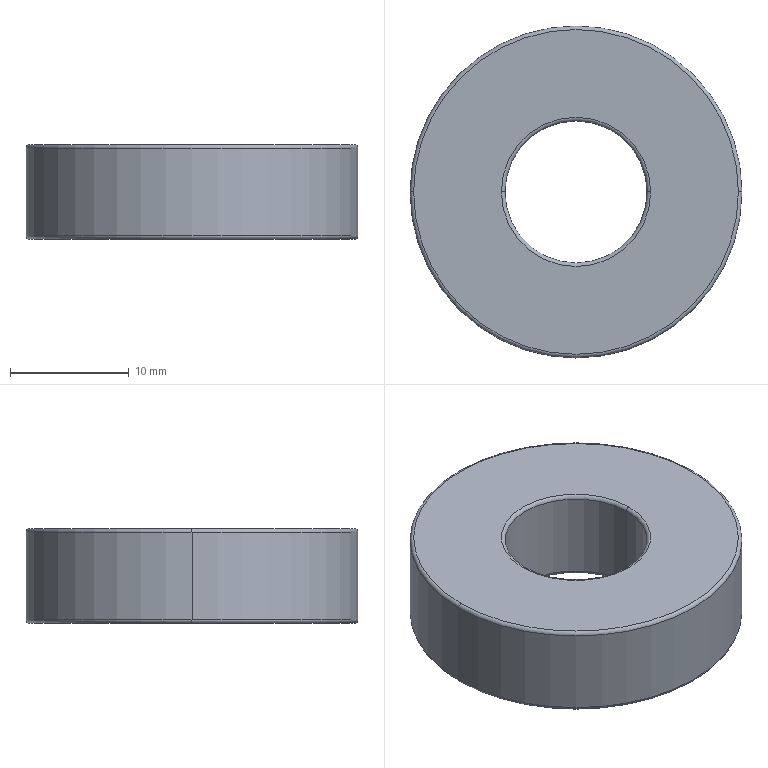Part | SolidWorks | features BaseBody 1 | 1 solid | 14 faces | box 28 x 28 x 8 mm | volume 4016 mm3 | torus 8 | cylinder 4 | plane 2 | commonest cylinder face diameters 12 x2 28 x2
STEP:
#1=CARTESIAN_POINT('',(-14.,0.,3.7));
#2=VERTEX_POINT('',#1);
#3=CARTESIAN_POINT('',(14.,0.,3.7));
#4=VERTEX_POINT('',#3);
#5=CARTESIAN_POINT('',(0.,0.,3.7));
#6=DIRECTION('',(0.,0.,-1.));
#7=DIRECTION('',(1.,0.,0.));
#8=AXIS2_PLACEMENT_3D('',#5,#6,#7);
#9=CIRCLE('',#8,14.);
#10=EDGE_CURVE('',#2,#4,#9,.T.);
#11=ORIENTED_EDGE('',*,*,#10,.F.);
#12=CARTESIAN_POINT('',(-13.7,0.,4.));
#13=VERTEX_POINT('',#12);
#14=CARTESIAN_POINT('',(-13.7,0.,3.7));
#15=DIRECTION('',(0.,1.,0.));
#16=DIRECTION('',(-1.,0.,0.));
#17=AXIS2_PLACEMENT_3D('',#14,#15,#16);
#18=CIRCLE('',#17,0.3);
#19=EDGE_CURVE('',#2,#13,#18,.T.);
#20=ORIENTED_EDGE('',*,*,#19,.T.);
#21=CARTESIAN_POINT('',(13.7,0.,4.));
#22=VERTEX_POINT('',#21);
#23=CARTESIAN_POINT('',(0.,0.,4.));
#24=DIRECTION('',(0.,0.,1.));
#25=DIRECTION('',(1.,0.,0.));
#26=AXIS2_PLACEMENT_3D('',#23,#24,#25);
#27=CIRCLE('',#26,13.7);
#28=EDGE_CURVE('',#22,#13,#27,.T.);
#29=ORIENTED_EDGE('',*,*,#28,.F.);
#30=CARTESIAN_POINT('',(13.7,0.,3.7));
#31=DIRECTION('',(0.,-1.,0.));
#32=DIRECTION('',(0.,0.,-1.));
#33=AXIS2_PLACEMENT_3D('',#30,#31,#32);
#34=CIRCLE('',#33,0.3);
#35=EDGE_CURVE('',#4,#22,#34,.T.);
#36=ORIENTED_EDGE('',*,*,#35,.F.);
#37=EDGE_LOOP('',(#11,#20,#29,#36));
#38=FACE_OUTER_BOUND('',#37,.T.);
#39=CARTESIAN_POINT('',(0.,0.,3.7));
#40=DIRECTION('',(0.,0.,1.));
#41=DIRECTION('',(1.,0.,0.));
#42=AXIS2_PLACEMENT_3D('',#39,#40,#41);
#43=TOROIDAL_SURFACE('',#42,13.7,0.3);
#44=ADVANCED_FACE('',(#38),#43,.T.);
#45=CARTESIAN_POINT('',(-13.7,0.,-4.));
#46=VERTEX_POINT('',#45);
#47=CARTESIAN_POINT('',(13.7,0.,-4.));
#48=VERTEX_POINT('',#47);
#49=CARTESIAN_POINT('',(0.,0.,-4.));
#50=DIRECTION('',(0.,0.,-1.));
#51=DIRECTION('',(1.,0.,0.));
#52=AXIS2_PLACEMENT_3D('',#49,#50,#51);
#53=CIRCLE('',#52,13.7);
#54=EDGE_CURVE('',#46,#48,#53,.T.);
#55=ORIENTED_EDGE('',*,*,#54,.F.);
#56=CARTESIAN_POINT('',(-14.,0.,-3.7));
#57=VERTEX_POINT('',#56);
#58=CARTESIAN_POINT('',(-13.7,0.,-3.7));
#59=DIRECTION('',(0.,1.,0.));
#60=DIRECTION('',(-1.,0.,0.));
#61=AXIS2_PLACEMENT_3D('',#58,#59,#60);
#62=CIRCLE('',#61,0.3);
#63=EDGE_CURVE('',#46,#57,#62,.T.);
#64=ORIENTED_EDGE('',*,*,#63,.T.);
#65=CARTESIAN_POINT('',(14.,0.,-3.7));
#66=VERTEX_POINT('',#65);
#67=CARTESIAN_POINT('',(0.,0.,-3.7));
#68=DIRECTION('',(0.,0.,1.));
#69=DIRECTION('',(1.,0.,0.));
#70=AXIS2_PLACEMENT_3D('',#67,#68,#69);
#71=CIRCLE('',#70,14.);
#72=EDGE_CURVE('',#66,#57,#71,.T.);
#73=ORIENTED_EDGE('',*,*,#72,.F.);
#74=CARTESIAN_POINT('',(13.7,0.,-3.7));
#75=DIRECTION('',(0.,-1.,0.));
#76=DIRECTION('',(0.,0.,-1.));
#77=AXIS2_PLACEMENT_3D('',#74,#75,#76);
#78=CIRCLE('',#77,0.3);
#79=EDGE_CURVE('',#48,#66,#78,.T.);
#80=ORIENTED_EDGE('',*,*,#79,.F.);
#81=EDGE_LOOP('',(#55,#64,#73,#80));
#82=FACE_OUTER_BOUND('',#81,.T.);
#83=CARTESIAN_POINT('',(0.,0.,-3.7));
#84=DIRECTION('',(0.,0.,1.));
#85=DIRECTION('',(1.,0.,0.));
#86=AXIS2_PLACEMENT_3D('',#83,#84,#85);
#87=TOROIDAL_SURFACE('',#86,13.7,0.3);
#88=ADVANCED_FACE('',(#82),#87,.T.);
#89=CARTESIAN_POINT('',(-6.3,0.,4.));
#90=VERTEX_POINT('',#89);
#91=CARTESIAN_POINT('',(6.3,0.,4.));
#92=VERTEX_POINT('',#91);
#93=CARTESIAN_POINT('',(0.,0.,4.));
#94=DIRECTION('',(0.,0.,-1.));
#95=DIRECTION('',(1.,0.,0.));
#96=AXIS2_PLACEMENT_3D('',#93,#94,#95);
#97=CIRCLE('',#96,6.3);
#98=EDGE_CURVE('',#90,#92,#97,.T.);
#99=ORIENTED_EDGE('',*,*,#98,.F.);
#100=CARTESIAN_POINT('',(-6.,0.,3.7));
#101=VERTEX_POINT('',#100);
#102=CARTESIAN_POINT('',(-6.3,0.,3.7));
#103=DIRECTION('',(0.,1.,0.));
#104=DIRECTION('',(-1.,0.,0.));
#105=AXIS2_PLACEMENT_3D('',#102,#103,#104);
#106=CIRCLE('',#105,0.3);
#107=EDGE_CURVE('',#90,#101,#106,.T.);
#108=ORIENTED_EDGE('',*,*,#107,.T.);
#109=CARTESIAN_POINT('',(6.,0.,3.7));
#110=VERTEX_POINT('',#109);
#111=CARTESIAN_POINT('',(0.,0.,3.7));
#112=DIRECTION('',(0.,0.,1.));
#113=DIRECTION('',(1.,0.,0.));
#114=AXIS2_PLACEMENT_3D('',#111,#112,#113);
#115=CIRCLE('',#114,6.);
#116=EDGE_CURVE('',#110,#101,#115,.T.);
#117=ORIENTED_EDGE('',*,*,#116,.F.);
#118=CARTESIAN_POINT('',(6.3,0.,3.7));
#119=DIRECTION('',(0.,-1.,0.));
#120=DIRECTION('',(0.,0.,-1.));
#121=AXIS2_PLACEMENT_3D('',#118,#119,#120);
#122=CIRCLE('',#121,0.3);
#123=EDGE_CURVE('',#92,#110,#122,.T.);
#124=ORIENTED_EDGE('',*,*,#123,.F.);
#125=EDGE_LOOP('',(#99,#108,#117,#124));
#126=FACE_OUTER_BOUND('',#125,.T.);
#127=CARTESIAN_POINT('',(0.,0.,3.7));
#128=DIRECTION('',(0.,0.,1.));
#129=DIRECTION('',(1.,0.,0.));
#130=AXIS2_PLACEMENT_3D('',#127,#128,#129);
#131=TOROIDAL_SURFACE('',#130,6.3,0.3);
#132=ADVANCED_FACE('',(#126),#131,.T.);
#133=CARTESIAN_POINT('',(-6.,0.,-3.7));
#134=VERTEX_POINT('',#133);
#135=CARTESIAN_POINT('',(6.,0.,-3.7));
#136=VERTEX_POINT('',#135);
#137=CARTESIAN_POINT('',(0.,0.,-3.7));
#138=DIRECTION('',(0.,0.,-1.));
#139=DIRECTION('',(1.,0.,0.));
#140=AXIS2_PLACEMENT_3D('',#137,#138,#139);
#141=CIRCLE('',#140,6.);
#142=EDGE_CURVE('',#134,#136,#141,.T.);
#143=ORIENTED_EDGE('',*,*,#142,.F.);
#144=CARTESIAN_POINT('',(-6.3,0.,-4.));
#145=VERTEX_POINT('',#144);
#146=CARTESIAN_POINT('',(-6.3,0.,-3.7));
#147=DIRECTION('',(0.,1.,0.));
#148=DIRECTION('',(-1.,0.,0.));
#149=AXIS2_PLACEMENT_3D('',#146,#147,#148);
#150=CIRCLE('',#149,0.3);
#151=EDGE_CURVE('',#134,#145,#150,.T.);
#152=ORIENTED_EDGE('',*,*,#151,.T.);
#153=CARTESIAN_POINT('',(6.3,0.,-4.));
#154=VERTEX_POINT('',#153);
#155=CARTESIAN_POINT('',(0.,0.,-4.));
#156=DIRECTION('',(0.,0.,1.));
#157=DIRECTION('',(1.,0.,0.));
#158=AXIS2_PLACEMENT_3D('',#155,#156,#157);
#159=CIRCLE('',#158,6.3);
#160=EDGE_CURVE('',#154,#145,#159,.T.);
#161=ORIENTED_EDGE('',*,*,#160,.F.);
#162=CARTESIAN_POINT('',(6.3,0.,-3.7));
#163=DIRECTION('',(0.,-1.,0.));
#164=DIRECTION('',(0.,0.,-1.));
#165=AXIS2_PLACEMENT_3D('',#162,#163,#164);
#166=CIRCLE('',#165,0.3);
#167=EDGE_CURVE('',#136,#154,#166,.T.);
#168=ORIENTED_EDGE('',*,*,#167,.F.);
#169=EDGE_LOOP('',(#143,#152,#161,#168));
#170=FACE_OUTER_BOUND('',#169,.T.);
#171=CARTESIAN_POINT('',(0.,0.,-3.7));
#172=DIRECTION('',(0.,0.,1.));
#173=DIRECTION('',(1.,0.,0.));
#174=AXIS2_PLACEMENT_3D('',#171,#172,#173);
#175=TOROIDAL_SURFACE('',#174,6.3,0.3);
#176=ADVANCED_FACE('',(#170),#175,.T.);
#177=CARTESIAN_POINT('',(0.,0.,3.7));
#178=DIRECTION('',(0.,0.,1.));
#179=DIRECTION('',(1.,0.,0.));
#180=AXIS2_PLACEMENT_3D('',#177,#178,#179);
#181=CIRCLE('',#180,6.);
#182=EDGE_CURVE('',#101,#110,#181,.T.);
#183=ORIENTED_EDGE('',*,*,#182,.T.);
#184=CARTESIAN_POINT('',(6.,0.,4.));
#185=DIRECTION('',(0.,0.,-1.));
#186=VECTOR('',#185,1000.);
#187=LINE('',#184,#186);
#188=EDGE_CURVE('',#110,#136,#187,.T.);
#189=ORIENTED_EDGE('',*,*,#188,.T.);
#190=CARTESIAN_POINT('',(0.,0.,-3.7));
#191=DIRECTION('',(0.,0.,-1.));
#192=DIRECTION('',(1.,0.,0.));
#193=AXIS2_PLACEMENT_3D('',#190,#191,#192);
#194=CIRCLE('',#193,6.);
#195=EDGE_CURVE('',#136,#134,#194,.T.);
#196=ORIENTED_EDGE('',*,*,#195,.T.);
#197=CARTESIAN_POINT('',(-6.,0.,4.));
#198=DIRECTION('',(0.,0.,-1.));
#199=VECTOR('',#198,1000.);
#200=LINE('',#197,#199);
#201=EDGE_CURVE('',#101,#134,#200,.T.);
#202=ORIENTED_EDGE('',*,*,#201,.F.);
#203=EDGE_LOOP('',(#183,#189,#196,#202));
#204=FACE_OUTER_BOUND('',#203,.T.);
#205=CARTESIAN_POINT('',(0.,0.,4.));
#206=DIRECTION('',(0.,0.,-1.));
#207=DIRECTION('',(-1.,0.,0.));
#208=AXIS2_PLACEMENT_3D('',#205,#206,#207);
#209=CYLINDRICAL_SURFACE('',#208,6.);
#210=ADVANCED_FACE('',(#204),#209,.F.);
#211=ORIENTED_EDGE('',*,*,#10,.T.);
#212=CARTESIAN_POINT('',(14.,0.,4.));
#213=DIRECTION('',(0.,0.,-1.));
#214=VECTOR('',#213,1000.);
#215=LINE('',#212,#214);
#216=EDGE_CURVE('',#4,#66,#215,.T.);
#217=ORIENTED_EDGE('',*,*,#216,.T.);
#218=ORIENTED_EDGE('',*,*,#72,.T.);
#219=CARTESIAN_POINT('',(-14.,0.,4.));
#220=DIRECTION('',(0.,0.,-1.));
#221=VECTOR('',#220,1000.);
#222=LINE('',#219,#221);
#223=EDGE_CURVE('',#2,#57,#222,.T.);
#224=ORIENTED_EDGE('',*,*,#223,.F.);
#225=EDGE_LOOP('',(#211,#217,#218,#224));
#226=FACE_OUTER_BOUND('',#225,.T.);
#227=CARTESIAN_POINT('',(0.,0.,4.));
#228=DIRECTION('',(0.,0.,-1.));
#229=DIRECTION('',(-1.,0.,0.));
#230=AXIS2_PLACEMENT_3D('',#227,#228,#229);
#231=CYLINDRICAL_SURFACE('',#230,14.);
#232=ADVANCED_FACE('',(#226),#231,.T.);
#233=ORIENTED_EDGE('',*,*,#160,.T.);
#234=CARTESIAN_POINT('',(0.,0.,-4.));
#235=DIRECTION('',(0.,0.,1.));
#236=DIRECTION('',(1.,0.,0.));
#237=AXIS2_PLACEMENT_3D('',#234,#235,#236);
#238=CIRCLE('',#237,6.3);
#239=EDGE_CURVE('',#145,#154,#238,.T.);
#240=ORIENTED_EDGE('',*,*,#239,.T.);
#241=EDGE_LOOP('',(#233,#240));
#242=FACE_BOUND('',#241,.T.);
#243=CARTESIAN_POINT('',(0.,0.,-4.));
#244=DIRECTION('',(0.,0.,-1.));
#245=DIRECTION('',(1.,0.,0.));
#246=AXIS2_PLACEMENT_3D('',#243,#244,#245);
#247=CIRCLE('',#246,13.7);
#248=EDGE_CURVE('',#48,#46,#247,.T.);
#249=ORIENTED_EDGE('',*,*,#248,.T.);
#250=ORIENTED_EDGE('',*,*,#54,.T.);
#251=EDGE_LOOP('',(#249,#250));
#252=FACE_OUTER_BOUND('',#251,.T.);
#253=CARTESIAN_POINT('',(0.,0.,-4.));
#254=DIRECTION('',(0.,0.,1.));
#255=DIRECTION('',(1.,0.,0.));
#256=AXIS2_PLACEMENT_3D('',#253,#254,#255);
#257=PLANE('',#256);
#258=ADVANCED_FACE('',(#242,#252),#257,.F.);
#259=CARTESIAN_POINT('',(0.,0.,4.));
#260=DIRECTION('',(0.,0.,-1.));
#261=DIRECTION('',(1.,0.,0.));
#262=AXIS2_PLACEMENT_3D('',#259,#260,#261);
#263=CIRCLE('',#262,6.3);
#264=EDGE_CURVE('',#92,#90,#263,.T.);
#265=ORIENTED_EDGE('',*,*,#264,.T.);
#266=ORIENTED_EDGE('',*,*,#98,.T.);
#267=EDGE_LOOP('',(#265,#266));
#268=FACE_BOUND('',#267,.T.);
#269=ORIENTED_EDGE('',*,*,#28,.T.);
#270=CARTESIAN_POINT('',(0.,0.,4.));
#271=DIRECTION('',(0.,0.,1.));
#272=DIRECTION('',(1.,0.,0.));
#273=AXIS2_PLACEMENT_3D('',#270,#271,#272);
#274=CIRCLE('',#273,13.7);
#275=EDGE_CURVE('',#13,#22,#274,.T.);
#276=ORIENTED_EDGE('',*,*,#275,.T.);
#277=EDGE_LOOP('',(#269,#276));
#278=FACE_OUTER_BOUND('',#277,.T.);
#279=CARTESIAN_POINT('',(0.,0.,4.));
#280=DIRECTION('',(0.,0.,1.));
#281=DIRECTION('',(1.,0.,0.));
#282=AXIS2_PLACEMENT_3D('',#279,#280,#281);
#283=PLANE('',#282);
#284=ADVANCED_FACE('',(#268,#278),#283,.T.);
#285=ORIENTED_EDGE('',*,*,#216,.F.);
#286=CARTESIAN_POINT('',(0.,0.,3.7));
#287=DIRECTION('',(0.,0.,-1.));
#288=DIRECTION('',(1.,0.,0.));
#289=AXIS2_PLACEMENT_3D('',#286,#287,#288);
#290=CIRCLE('',#289,14.);
#291=EDGE_CURVE('',#4,#2,#290,.T.);
#292=ORIENTED_EDGE('',*,*,#291,.T.);
#293=ORIENTED_EDGE('',*,*,#223,.T.);
#294=CARTESIAN_POINT('',(0.,0.,-3.7));
#295=DIRECTION('',(0.,0.,1.));
#296=DIRECTION('',(1.,0.,0.));
#297=AXIS2_PLACEMENT_3D('',#294,#295,#296);
#298=CIRCLE('',#297,14.);
#299=EDGE_CURVE('',#57,#66,#298,.T.);
#300=ORIENTED_EDGE('',*,*,#299,.T.);
#301=EDGE_LOOP('',(#285,#292,#293,#300));
#302=FACE_OUTER_BOUND('',#301,.T.);
#303=CARTESIAN_POINT('',(0.,0.,4.));
#304=DIRECTION('',(0.,0.,-1.));
#305=DIRECTION('',(-1.,0.,0.));
#306=AXIS2_PLACEMENT_3D('',#303,#304,#305);
#307=CYLINDRICAL_SURFACE('',#306,14.);
#308=ADVANCED_FACE('',(#302),#307,.T.);
#309=ORIENTED_EDGE('',*,*,#188,.F.);
#310=ORIENTED_EDGE('',*,*,#116,.T.);
#311=ORIENTED_EDGE('',*,*,#201,.T.);
#312=ORIENTED_EDGE('',*,*,#142,.T.);
#313=EDGE_LOOP('',(#309,#310,#311,#312));
#314=FACE_OUTER_BOUND('',#313,.T.);
#315=CARTESIAN_POINT('',(0.,0.,4.));
#316=DIRECTION('',(0.,0.,-1.));
#317=DIRECTION('',(-1.,0.,0.));
#318=AXIS2_PLACEMENT_3D('',#315,#316,#317);
#319=CYLINDRICAL_SURFACE('',#318,6.);
#320=ADVANCED_FACE('',(#314),#319,.F.);
#321=ORIENTED_EDGE('',*,*,#151,.F.);
#322=ORIENTED_EDGE('',*,*,#195,.F.);
#323=ORIENTED_EDGE('',*,*,#167,.T.);
#324=ORIENTED_EDGE('',*,*,#239,.F.);
#325=EDGE_LOOP('',(#321,#322,#323,#324));
#326=FACE_OUTER_BOUND('',#325,.T.);
#327=CARTESIAN_POINT('',(0.,0.,-3.7));
#328=DIRECTION('',(0.,0.,1.));
#329=DIRECTION('',(1.,0.,0.));
#330=AXIS2_PLACEMENT_3D('',#327,#328,#329);
#331=TOROIDAL_SURFACE('',#330,6.3,0.3);
#332=ADVANCED_FACE('',(#326),#331,.T.);
#333=ORIENTED_EDGE('',*,*,#107,.F.);
#334=ORIENTED_EDGE('',*,*,#264,.F.);
#335=ORIENTED_EDGE('',*,*,#123,.T.);
#336=ORIENTED_EDGE('',*,*,#182,.F.);
#337=EDGE_LOOP('',(#333,#334,#335,#336));
#338=FACE_OUTER_BOUND('',#337,.T.);
#339=CARTESIAN_POINT('',(0.,0.,3.7));
#340=DIRECTION('',(0.,0.,1.));
#341=DIRECTION('',(1.,0.,0.));
#342=AXIS2_PLACEMENT_3D('',#339,#340,#341);
#343=TOROIDAL_SURFACE('',#342,6.3,0.3);
#344=ADVANCED_FACE('',(#338),#343,.T.);
#345=ORIENTED_EDGE('',*,*,#63,.F.);
#346=ORIENTED_EDGE('',*,*,#248,.F.);
#347=ORIENTED_EDGE('',*,*,#79,.T.);
#348=ORIENTED_EDGE('',*,*,#299,.F.);
#349=EDGE_LOOP('',(#345,#346,#347,#348));
#350=FACE_OUTER_BOUND('',#349,.T.);
#351=CARTESIAN_POINT('',(0.,0.,-3.7));
#352=DIRECTION('',(0.,0.,1.));
#353=DIRECTION('',(1.,0.,0.));
#354=AXIS2_PLACEMENT_3D('',#351,#352,#353);
#355=TOROIDAL_SURFACE('',#354,13.7,0.3);
#356=ADVANCED_FACE('',(#350),#355,.T.);
#357=ORIENTED_EDGE('',*,*,#19,.F.);
#358=ORIENTED_EDGE('',*,*,#291,.F.);
#359=ORIENTED_EDGE('',*,*,#35,.T.);
#360=ORIENTED_EDGE('',*,*,#275,.F.);
#361=EDGE_LOOP('',(#357,#358,#359,#360));
#362=FACE_OUTER_BOUND('',#361,.T.);
#363=CARTESIAN_POINT('',(0.,0.,3.7));
#364=DIRECTION('',(0.,0.,1.));
#365=DIRECTION('',(1.,0.,0.));
#366=AXIS2_PLACEMENT_3D('',#363,#364,#365);
#367=TOROIDAL_SURFACE('',#366,13.7,0.3);
#368=ADVANCED_FACE('',(#362),#367,.T.);
#369=CLOSED_SHELL('',(#44,#88,#132,#176,#210,#232,#258,#284,#308,#320,#332,#344,#356,#368));
#370=MANIFOLD_SOLID_BREP('',#369);
#371=CARTESIAN_POINT('',(0.,0.,0.));
#372=DIRECTION('',(0.,0.,1.));
#373=DIRECTION('',(1.,0.,0.));
#374=AXIS2_PLACEMENT_3D('',#371,#372,#373);
#375=(LENGTH_UNIT()NAMED_UNIT(*)SI_UNIT(.MILLI.,.METRE.));
#376=UNCERTAINTY_MEASURE_WITH_UNIT(LENGTH_MEASURE(0.00001),#375,'','');
#377=(NAMED_UNIT(*)PLANE_ANGLE_UNIT()SI_UNIT($,.RADIAN.));
#378=(NAMED_UNIT(*)SI_UNIT($,.STERADIAN.)SOLID_ANGLE_UNIT());
#379=(GEOMETRIC_REPRESENTATION_CONTEXT(3)GLOBAL_UNCERTAINTY_ASSIGNED_CONTEXT((#376))GLOBAL_UNIT_ASSIGNED_CONTEXT((#375,#377,#378))REPRESENTATION_CONTEXT('',''));
#380=ADVANCED_BREP_SHAPE_REPRESENTATION('',(#370,#374),#379);